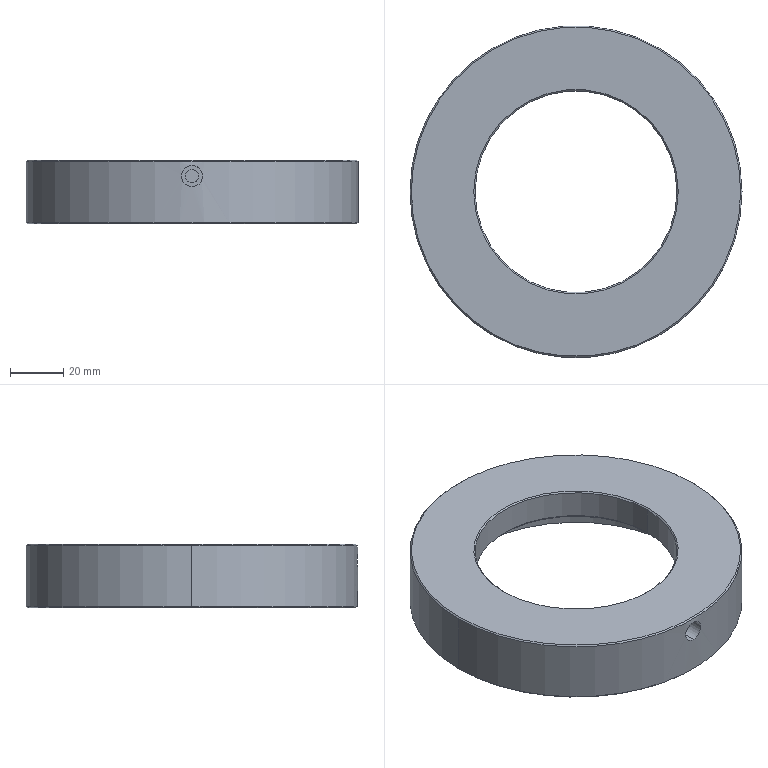Part | STEP file | 2093 Limit side plate B2 | 1 solid | 38 faces | box 125 x 125 x 24 mm | volume 136649 mm3 | cylinder 18 | cone 16 | plane 4 | commonest cylinder face diameters 3.3 x8 5 x2 8 x2 76 x2 104 x2 125 x2